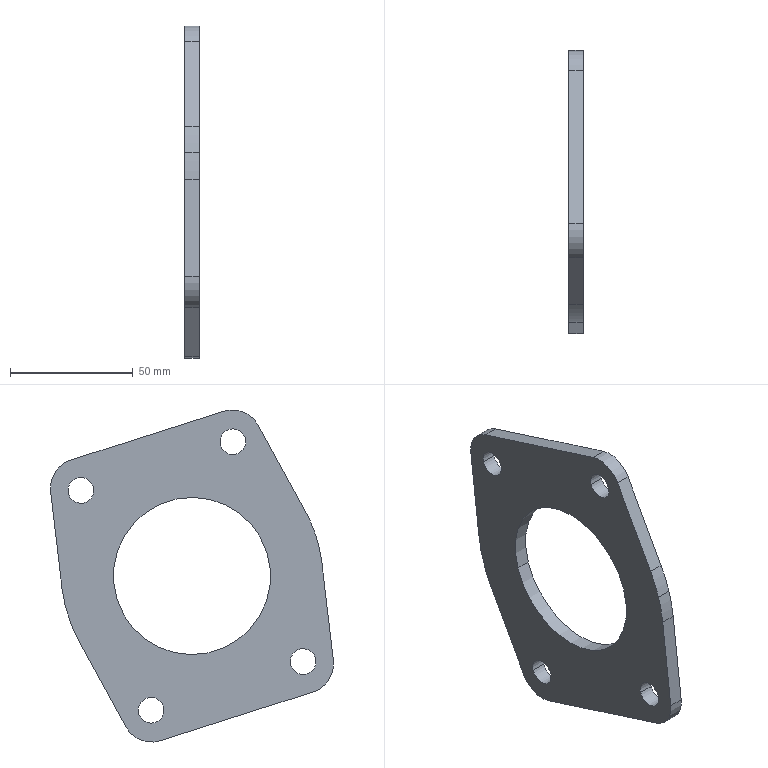Part | NX | features BREP 1 | 1 solid | 25 faces | box 6 x 115.344 x 135.296 mm | volume 47647 mm3 | cylinder 17 | plane 8 | commonest cylinder face diameters 10.5 x8 24 x4 120 x3 64 x2
STEP:
#1=CARTESIAN_POINT('',(-624.265,-30.481,9.741));
#2=VERTEX_POINT('',#1);
#3=CARTESIAN_POINT('',(-624.265,30.481,-9.741));
#4=VERTEX_POINT('',#3);
#5=CARTESIAN_POINT('',(-624.265,0.,0.));
#6=DIRECTION('',(1.,0.,0.));
#7=DIRECTION('',(0.,-0.9525,0.3044));
#8=AXIS2_PLACEMENT_3D('',#5,#6,#7);
#9=CIRCLE('',#8,32.);
#10=EDGE_CURVE('',#2,#4,#9,.T.);
#11=ORIENTED_EDGE('',*,*,#10,.T.);
#12=CARTESIAN_POINT('',(-630.265,30.481,-9.741));
#13=VERTEX_POINT('',#12);
#14=CARTESIAN_POINT('',(-624.265,30.481,-9.741));
#15=DIRECTION('',(-1.,0.,0.));
#16=VECTOR('',#15,1000.);
#17=LINE('',#14,#16);
#18=EDGE_CURVE('',#13,#4,#17,.F.);
#19=ORIENTED_EDGE('',*,*,#18,.F.);
#20=CARTESIAN_POINT('',(-630.265,-30.481,9.741));
#21=VERTEX_POINT('',#20);
#22=CARTESIAN_POINT('',(-630.265,0.,0.));
#23=DIRECTION('',(1.,0.,0.));
#24=DIRECTION('',(0.,-0.9525,0.3044));
#25=AXIS2_PLACEMENT_3D('',#22,#23,#24);
#26=CIRCLE('',#25,32.);
#27=EDGE_CURVE('',#21,#13,#26,.T.);
#28=ORIENTED_EDGE('',*,*,#27,.F.);
#29=CARTESIAN_POINT('',(-624.265,-30.481,9.741));
#30=DIRECTION('',(-1.,0.,0.));
#31=VECTOR('',#30,1000.);
#32=LINE('',#29,#31);
#33=EDGE_CURVE('',#21,#2,#32,.F.);
#34=ORIENTED_EDGE('',*,*,#33,.T.);
#35=EDGE_LOOP('',(#11,#19,#28,#34));
#36=FACE_BOUND('',#35,.T.);
#37=CARTESIAN_POINT('',(-624.265,0.,0.));
#38=DIRECTION('',(-1.,0.,0.));
#39=DIRECTION('',(0.,0.9525,-0.3044));
#40=AXIS2_PLACEMENT_3D('',#37,#38,#39);
#41=CYLINDRICAL_SURFACE('',#40,32.);
#42=ADVANCED_FACE('',(#36),#41,.F.);
#43=CARTESIAN_POINT('',(-624.265,40.264,36.474));
#44=VERTEX_POINT('',#43);
#45=CARTESIAN_POINT('',(-624.265,50.266,33.278));
#46=VERTEX_POINT('',#45);
#47=CARTESIAN_POINT('',(-624.265,45.265,34.876));
#48=DIRECTION('',(1.,0.,0.));
#49=DIRECTION('',(0.,-0.9525,0.3044));
#50=AXIS2_PLACEMENT_3D('',#47,#48,#49);
#51=CIRCLE('',#50,5.25);
#52=EDGE_CURVE('',#44,#46,#51,.T.);
#53=ORIENTED_EDGE('',*,*,#52,.T.);
#54=CARTESIAN_POINT('',(-630.265,50.266,33.278));
#55=VERTEX_POINT('',#54);
#56=CARTESIAN_POINT('',(-624.265,50.266,33.278));
#57=DIRECTION('',(-1.,0.,0.));
#58=VECTOR('',#57,1000.);
#59=LINE('',#56,#58);
#60=EDGE_CURVE('',#55,#46,#59,.F.);
#61=ORIENTED_EDGE('',*,*,#60,.F.);
#62=CARTESIAN_POINT('',(-630.265,40.264,36.474));
#63=VERTEX_POINT('',#62);
#64=CARTESIAN_POINT('',(-630.265,45.265,34.876));
#65=DIRECTION('',(1.,0.,0.));
#66=DIRECTION('',(0.,-0.9525,0.3044));
#67=AXIS2_PLACEMENT_3D('',#64,#65,#66);
#68=CIRCLE('',#67,5.25);
#69=EDGE_CURVE('',#63,#55,#68,.T.);
#70=ORIENTED_EDGE('',*,*,#69,.F.);
#71=CARTESIAN_POINT('',(-624.265,40.264,36.474));
#72=DIRECTION('',(-1.,0.,0.));
#73=VECTOR('',#72,1000.);
#74=LINE('',#71,#73);
#75=EDGE_CURVE('',#63,#44,#74,.F.);
#76=ORIENTED_EDGE('',*,*,#75,.T.);
#77=EDGE_LOOP('',(#53,#61,#70,#76));
#78=FACE_BOUND('',#77,.T.);
#79=CARTESIAN_POINT('',(-624.265,45.265,34.876));
#80=DIRECTION('',(-1.,0.,0.));
#81=DIRECTION('',(0.,0.9525,-0.3044));
#82=AXIS2_PLACEMENT_3D('',#79,#80,#81);
#83=CYLINDRICAL_SURFACE('',#82,5.25);
#84=ADVANCED_FACE('',(#78),#83,.F.);
#85=CARTESIAN_POINT('',(-624.265,-21.651,56.261));
#86=VERTEX_POINT('',#85);
#87=CARTESIAN_POINT('',(-624.265,-11.65,53.065));
#88=VERTEX_POINT('',#87);
#89=CARTESIAN_POINT('',(-624.265,-16.65,54.663));
#90=DIRECTION('',(1.,0.,0.));
#91=DIRECTION('',(0.,-0.9525,0.3044));
#92=AXIS2_PLACEMENT_3D('',#89,#90,#91);
#93=CIRCLE('',#92,5.25);
#94=EDGE_CURVE('',#86,#88,#93,.T.);
#95=ORIENTED_EDGE('',*,*,#94,.T.);
#96=CARTESIAN_POINT('',(-630.265,-11.65,53.065));
#97=VERTEX_POINT('',#96);
#98=CARTESIAN_POINT('',(-624.265,-11.65,53.065));
#99=DIRECTION('',(-1.,0.,0.));
#100=VECTOR('',#99,1000.);
#101=LINE('',#98,#100);
#102=EDGE_CURVE('',#97,#88,#101,.F.);
#103=ORIENTED_EDGE('',*,*,#102,.F.);
#104=CARTESIAN_POINT('',(-630.265,-21.651,56.261));
#105=VERTEX_POINT('',#104);
#106=CARTESIAN_POINT('',(-630.265,-16.65,54.663));
#107=DIRECTION('',(1.,0.,0.));
#108=DIRECTION('',(0.,-0.9525,0.3044));
#109=AXIS2_PLACEMENT_3D('',#106,#107,#108);
#110=CIRCLE('',#109,5.25);
#111=EDGE_CURVE('',#105,#97,#110,.T.);
#112=ORIENTED_EDGE('',*,*,#111,.F.);
#113=CARTESIAN_POINT('',(-624.265,-21.651,56.261));
#114=DIRECTION('',(-1.,0.,0.));
#115=VECTOR('',#114,1000.);
#116=LINE('',#113,#115);
#117=EDGE_CURVE('',#105,#86,#116,.F.);
#118=ORIENTED_EDGE('',*,*,#117,.T.);
#119=EDGE_LOOP('',(#95,#103,#112,#118));
#120=FACE_BOUND('',#119,.T.);
#121=CARTESIAN_POINT('',(-624.265,-16.65,54.663));
#122=DIRECTION('',(-1.,0.,0.));
#123=DIRECTION('',(0.,0.9525,-0.3044));
#124=AXIS2_PLACEMENT_3D('',#121,#122,#123);
#125=CYLINDRICAL_SURFACE('',#124,5.25);
#126=ADVANCED_FACE('',(#120),#125,.F.);
#127=CARTESIAN_POINT('',(-624.265,-50.266,-33.278));
#128=VERTEX_POINT('',#127);
#129=CARTESIAN_POINT('',(-624.265,-40.264,-36.474));
#130=VERTEX_POINT('',#129);
#131=CARTESIAN_POINT('',(-624.265,-45.265,-34.876));
#132=DIRECTION('',(1.,0.,0.));
#133=DIRECTION('',(0.,-0.9525,0.3044));
#134=AXIS2_PLACEMENT_3D('',#131,#132,#133);
#135=CIRCLE('',#134,5.25);
#136=EDGE_CURVE('',#128,#130,#135,.T.);
#137=ORIENTED_EDGE('',*,*,#136,.T.);
#138=CARTESIAN_POINT('',(-630.265,-40.264,-36.474));
#139=VERTEX_POINT('',#138);
#140=CARTESIAN_POINT('',(-624.265,-40.264,-36.474));
#141=DIRECTION('',(-1.,0.,0.));
#142=VECTOR('',#141,1000.);
#143=LINE('',#140,#142);
#144=EDGE_CURVE('',#139,#130,#143,.F.);
#145=ORIENTED_EDGE('',*,*,#144,.F.);
#146=CARTESIAN_POINT('',(-630.265,-50.266,-33.278));
#147=VERTEX_POINT('',#146);
#148=CARTESIAN_POINT('',(-630.265,-45.265,-34.876));
#149=DIRECTION('',(1.,0.,0.));
#150=DIRECTION('',(0.,-0.9525,0.3044));
#151=AXIS2_PLACEMENT_3D('',#148,#149,#150);
#152=CIRCLE('',#151,5.25);
#153=EDGE_CURVE('',#147,#139,#152,.T.);
#154=ORIENTED_EDGE('',*,*,#153,.F.);
#155=CARTESIAN_POINT('',(-624.265,-50.266,-33.278));
#156=DIRECTION('',(-1.,0.,0.));
#157=VECTOR('',#156,1000.);
#158=LINE('',#155,#157);
#159=EDGE_CURVE('',#147,#128,#158,.F.);
#160=ORIENTED_EDGE('',*,*,#159,.T.);
#161=EDGE_LOOP('',(#137,#145,#154,#160));
#162=FACE_BOUND('',#161,.T.);
#163=CARTESIAN_POINT('',(-624.265,-45.265,-34.876));
#164=DIRECTION('',(-1.,0.,0.));
#165=DIRECTION('',(0.,0.9525,-0.3044));
#166=AXIS2_PLACEMENT_3D('',#163,#164,#165);
#167=CYLINDRICAL_SURFACE('',#166,5.25);
#168=ADVANCED_FACE('',(#162),#167,.F.);
#169=CARTESIAN_POINT('',(-624.265,11.65,-53.065));
#170=VERTEX_POINT('',#169);
#171=CARTESIAN_POINT('',(-624.265,21.651,-56.261));
#172=VERTEX_POINT('',#171);
#173=CARTESIAN_POINT('',(-624.265,16.65,-54.663));
#174=DIRECTION('',(1.,0.,0.));
#175=DIRECTION('',(0.,-0.9525,0.3044));
#176=AXIS2_PLACEMENT_3D('',#173,#174,#175);
#177=CIRCLE('',#176,5.25);
#178=EDGE_CURVE('',#170,#172,#177,.T.);
#179=ORIENTED_EDGE('',*,*,#178,.T.);
#180=CARTESIAN_POINT('',(-630.265,21.651,-56.261));
#181=VERTEX_POINT('',#180);
#182=CARTESIAN_POINT('',(-624.265,21.651,-56.261));
#183=DIRECTION('',(-1.,0.,0.));
#184=VECTOR('',#183,1000.);
#185=LINE('',#182,#184);
#186=EDGE_CURVE('',#181,#172,#185,.F.);
#187=ORIENTED_EDGE('',*,*,#186,.F.);
#188=CARTESIAN_POINT('',(-630.265,11.65,-53.065));
#189=VERTEX_POINT('',#188);
#190=CARTESIAN_POINT('',(-630.265,16.65,-54.663));
#191=DIRECTION('',(1.,0.,0.));
#192=DIRECTION('',(0.,-0.9525,0.3044));
#193=AXIS2_PLACEMENT_3D('',#190,#191,#192);
#194=CIRCLE('',#193,5.25);
#195=EDGE_CURVE('',#189,#181,#194,.T.);
#196=ORIENTED_EDGE('',*,*,#195,.F.);
#197=CARTESIAN_POINT('',(-624.265,11.65,-53.065));
#198=DIRECTION('',(-1.,0.,0.));
#199=VECTOR('',#198,1000.);
#200=LINE('',#197,#199);
#201=EDGE_CURVE('',#189,#170,#200,.F.);
#202=ORIENTED_EDGE('',*,*,#201,.T.);
#203=EDGE_LOOP('',(#179,#187,#196,#202));
#204=FACE_BOUND('',#203,.T.);
#205=CARTESIAN_POINT('',(-624.265,16.65,-54.663));
#206=DIRECTION('',(-1.,0.,0.));
#207=DIRECTION('',(0.,0.9525,-0.3044));
#208=AXIS2_PLACEMENT_3D('',#205,#206,#207);
#209=CYLINDRICAL_SURFACE('',#208,5.25);
#210=ADVANCED_FACE('',(#204),#209,.F.);
#211=CARTESIAN_POINT('',(-624.265,-50.523,16.146));
#212=VERTEX_POINT('',#211);
#213=CARTESIAN_POINT('',(-624.265,-52.958,4.905));
#214=VERTEX_POINT('',#213);
#215=CARTESIAN_POINT('',(-624.265,6.63,-2.119));
#216=DIRECTION('',(1.,0.,0.));
#217=DIRECTION('',(0.,0.9525,-0.3044));
#218=AXIS2_PLACEMENT_3D('',#215,#216,#217);
#219=CIRCLE('',#218,60.);
#220=EDGE_CURVE('',#212,#214,#219,.T.);
#221=ORIENTED_EDGE('',*,*,#220,.F.);
#222=CARTESIAN_POINT('',(-630.265,-50.523,16.146));
#223=VERTEX_POINT('',#222);
#224=CARTESIAN_POINT('',(-624.265,-50.523,16.146));
#225=DIRECTION('',(-1.,0.,0.));
#226=VECTOR('',#225,1000.);
#227=LINE('',#224,#226);
#228=EDGE_CURVE('',#212,#223,#227,.T.);
#229=ORIENTED_EDGE('',*,*,#228,.T.);
#230=CARTESIAN_POINT('',(-630.265,-52.958,4.905));
#231=VERTEX_POINT('',#230);
#232=CARTESIAN_POINT('',(-630.265,6.63,-2.119));
#233=DIRECTION('',(1.,0.,0.));
#234=DIRECTION('',(0.,0.9525,-0.3044));
#235=AXIS2_PLACEMENT_3D('',#232,#233,#234);
#236=CIRCLE('',#235,60.);
#237=EDGE_CURVE('',#223,#231,#236,.T.);
#238=ORIENTED_EDGE('',*,*,#237,.T.);
#239=CARTESIAN_POINT('',(-624.265,-52.958,4.905));
#240=DIRECTION('',(-1.,0.,0.));
#241=VECTOR('',#240,1000.);
#242=LINE('',#239,#241);
#243=EDGE_CURVE('',#214,#231,#242,.T.);
#244=ORIENTED_EDGE('',*,*,#243,.F.);
#245=EDGE_LOOP('',(#221,#229,#238,#244));
#246=FACE_BOUND('',#245,.T.);
#247=CARTESIAN_POINT('',(-624.265,6.63,-2.119));
#248=DIRECTION('',(-1.,0.,0.));
#249=DIRECTION('',(0.,0.9525,-0.3044));
#250=AXIS2_PLACEMENT_3D('',#247,#248,#249);
#251=CYLINDRICAL_SURFACE('',#250,60.);
#252=ADVANCED_FACE('',(#246),#251,.T.);
#253=ORIENTED_EDGE('',*,*,#52,.F.);
#254=CARTESIAN_POINT('',(-624.265,45.265,34.876));
#255=DIRECTION('',(1.,0.,0.));
#256=DIRECTION('',(0.,-0.9525,0.3044));
#257=AXIS2_PLACEMENT_3D('',#254,#255,#256);
#258=CIRCLE('',#257,5.25);
#259=EDGE_CURVE('',#46,#44,#258,.T.);
#260=ORIENTED_EDGE('',*,*,#259,.F.);
#261=EDGE_LOOP('',(#253,#260));
#262=FACE_BOUND('',#261,.T.);
#263=ORIENTED_EDGE('',*,*,#136,.F.);
#264=CARTESIAN_POINT('',(-624.265,-45.265,-34.876));
#265=DIRECTION('',(1.,0.,0.));
#266=DIRECTION('',(0.,-0.9525,0.3044));
#267=AXIS2_PLACEMENT_3D('',#264,#265,#266);
#268=CIRCLE('',#267,5.25);
#269=EDGE_CURVE('',#130,#128,#268,.T.);
#270=ORIENTED_EDGE('',*,*,#269,.F.);
#271=EDGE_LOOP('',(#263,#270));
#272=FACE_BOUND('',#271,.T.);
#273=CARTESIAN_POINT('',(-624.265,-57.59,-34.391));
#274=VERTEX_POINT('',#273);
#275=CARTESIAN_POINT('',(-624.265,-49.325,-47.226));
#276=VERTEX_POINT('',#275);
#277=CARTESIAN_POINT('',(-624.265,-45.672,-35.796));
#278=DIRECTION('',(1.,0.,0.));
#279=DIRECTION('',(0.,0.9525,-0.3044));
#280=AXIS2_PLACEMENT_3D('',#277,#278,#279);
#281=CIRCLE('',#280,12.);
#282=EDGE_CURVE('',#274,#276,#281,.T.);
#283=ORIENTED_EDGE('',*,*,#282,.T.);
#284=CARTESIAN_POINT('',(-624.265,12.796,-67.079));
#285=VERTEX_POINT('',#284);
#286=CARTESIAN_POINT('',(-624.265,-49.325,-47.226));
#287=DIRECTION('',(0.,0.9525,-0.3044));
#288=VECTOR('',#287,1000.);
#289=LINE('',#286,#288);
#290=EDGE_CURVE('',#276,#285,#289,.T.);
#291=ORIENTED_EDGE('',*,*,#290,.T.);
#292=CARTESIAN_POINT('',(-624.265,26.972,-61.415));
#293=VERTEX_POINT('',#292);
#294=CARTESIAN_POINT('',(-624.265,16.449,-55.648));
#295=DIRECTION('',(1.,0.,0.));
#296=DIRECTION('',(0.,0.9525,-0.3044));
#297=AXIS2_PLACEMENT_3D('',#294,#295,#296);
#298=CIRCLE('',#297,12.);
#299=EDGE_CURVE('',#285,#293,#298,.T.);
#300=ORIENTED_EDGE('',*,*,#299,.T.);
#301=CARTESIAN_POINT('',(-624.265,45.988,-26.715));
#302=VERTEX_POINT('',#301);
#303=CARTESIAN_POINT('',(-624.265,26.972,-61.415));
#304=DIRECTION('',(0.,0.4806,0.877));
#305=VECTOR('',#304,1000.);
#306=LINE('',#303,#305);
#307=EDGE_CURVE('',#293,#302,#306,.T.);
#308=ORIENTED_EDGE('',*,*,#307,.T.);
#309=CARTESIAN_POINT('',(-624.265,52.958,-4.905));
#310=VERTEX_POINT('',#309);
#311=CARTESIAN_POINT('',(-624.265,-6.63,2.119));
#312=DIRECTION('',(1.,0.,0.));
#313=DIRECTION('',(0.,0.9525,-0.3044));
#314=AXIS2_PLACEMENT_3D('',#311,#312,#313);
#315=CIRCLE('',#314,60.);
#316=EDGE_CURVE('',#302,#310,#315,.T.);
#317=ORIENTED_EDGE('',*,*,#316,.T.);
#318=CARTESIAN_POINT('',(-624.265,57.59,34.391));
#319=VERTEX_POINT('',#318);
#320=CARTESIAN_POINT('',(-624.265,52.958,-4.905));
#321=DIRECTION('',(0.,0.1171,0.9931));
#322=VECTOR('',#321,1000.);
#323=LINE('',#320,#322);
#324=EDGE_CURVE('',#310,#319,#323,.T.);
#325=ORIENTED_EDGE('',*,*,#324,.T.);
#326=CARTESIAN_POINT('',(-624.265,49.325,47.226));
#327=VERTEX_POINT('',#326);
#328=CARTESIAN_POINT('',(-624.265,45.672,35.796));
#329=DIRECTION('',(1.,0.,0.));
#330=DIRECTION('',(0.,0.9525,-0.3044));
#331=AXIS2_PLACEMENT_3D('',#328,#329,#330);
#332=CIRCLE('',#331,12.);
#333=EDGE_CURVE('',#319,#327,#332,.T.);
#334=ORIENTED_EDGE('',*,*,#333,.T.);
#335=CARTESIAN_POINT('',(-624.265,-12.796,67.079));
#336=VERTEX_POINT('',#335);
#337=CARTESIAN_POINT('',(-624.265,49.325,47.226));
#338=DIRECTION('',(0.,-0.9525,0.3044));
#339=VECTOR('',#338,1000.);
#340=LINE('',#337,#339);
#341=EDGE_CURVE('',#327,#336,#340,.T.);
#342=ORIENTED_EDGE('',*,*,#341,.T.);
#343=CARTESIAN_POINT('',(-624.265,-26.972,61.415));
#344=VERTEX_POINT('',#343);
#345=CARTESIAN_POINT('',(-624.265,-16.449,55.648));
#346=DIRECTION('',(1.,0.,0.));
#347=DIRECTION('',(0.,0.9525,-0.3044));
#348=AXIS2_PLACEMENT_3D('',#345,#346,#347);
#349=CIRCLE('',#348,12.);
#350=EDGE_CURVE('',#336,#344,#349,.T.);
#351=ORIENTED_EDGE('',*,*,#350,.T.);
#352=CARTESIAN_POINT('',(-624.265,-45.988,26.715));
#353=VERTEX_POINT('',#352);
#354=CARTESIAN_POINT('',(-624.265,-26.972,61.415));
#355=DIRECTION('',(0.,-0.4806,-0.877));
#356=VECTOR('',#355,1000.);
#357=LINE('',#354,#356);
#358=EDGE_CURVE('',#344,#353,#357,.T.);
#359=ORIENTED_EDGE('',*,*,#358,.T.);
#360=CARTESIAN_POINT('',(-624.265,6.63,-2.119));
#361=DIRECTION('',(1.,0.,0.));
#362=DIRECTION('',(0.,0.9525,-0.3044));
#363=AXIS2_PLACEMENT_3D('',#360,#361,#362);
#364=CIRCLE('',#363,60.);
#365=EDGE_CURVE('',#353,#212,#364,.T.);
#366=ORIENTED_EDGE('',*,*,#365,.T.);
#367=ORIENTED_EDGE('',*,*,#220,.T.);
#368=CARTESIAN_POINT('',(-624.265,-52.958,4.905));
#369=DIRECTION('',(0.,-0.1171,-0.9931));
#370=VECTOR('',#369,1000.);
#371=LINE('',#368,#370);
#372=EDGE_CURVE('',#214,#274,#371,.T.);
#373=ORIENTED_EDGE('',*,*,#372,.T.);
#374=EDGE_LOOP('',(#283,#291,#300,#308,#317,#325,#334,#342,#351,#359,#366,#367,#373));
#375=FACE_BOUND('',#374,.T.);
#376=ORIENTED_EDGE('',*,*,#178,.F.);
#377=CARTESIAN_POINT('',(-624.265,16.65,-54.663));
#378=DIRECTION('',(1.,0.,0.));
#379=DIRECTION('',(0.,-0.9525,0.3044));
#380=AXIS2_PLACEMENT_3D('',#377,#378,#379);
#381=CIRCLE('',#380,5.25);
#382=EDGE_CURVE('',#172,#170,#381,.T.);
#383=ORIENTED_EDGE('',*,*,#382,.F.);
#384=EDGE_LOOP('',(#376,#383));
#385=FACE_BOUND('',#384,.T.);
#386=ORIENTED_EDGE('',*,*,#94,.F.);
#387=CARTESIAN_POINT('',(-624.265,-16.65,54.663));
#388=DIRECTION('',(1.,0.,0.));
#389=DIRECTION('',(0.,-0.9525,0.3044));
#390=AXIS2_PLACEMENT_3D('',#387,#388,#389);
#391=CIRCLE('',#390,5.25);
#392=EDGE_CURVE('',#88,#86,#391,.T.);
#393=ORIENTED_EDGE('',*,*,#392,.F.);
#394=EDGE_LOOP('',(#386,#393));
#395=FACE_BOUND('',#394,.T.);
#396=ORIENTED_EDGE('',*,*,#10,.F.);
#397=CARTESIAN_POINT('',(-624.265,0.,0.));
#398=DIRECTION('',(1.,0.,0.));
#399=DIRECTION('',(0.,-0.9525,0.3044));
#400=AXIS2_PLACEMENT_3D('',#397,#398,#399);
#401=CIRCLE('',#400,32.);
#402=EDGE_CURVE('',#4,#2,#401,.T.);
#403=ORIENTED_EDGE('',*,*,#402,.F.);
#404=EDGE_LOOP('',(#396,#403));
#405=FACE_BOUND('',#404,.T.);
#406=CARTESIAN_POINT('',(-624.265,-45.672,-35.796));
#407=DIRECTION('',(1.,0.,0.));
#408=DIRECTION('',(0.,-0.9525,0.3044));
#409=AXIS2_PLACEMENT_3D('',#406,#407,#408);
#410=PLANE('',#409);
#411=ADVANCED_FACE('',(#262,#272,#375,#385,#395,#405),#410,.T.);
#412=CARTESIAN_POINT('',(-630.265,-57.59,-34.391));
#413=VERTEX_POINT('',#412);
#414=CARTESIAN_POINT('',(-630.265,-49.325,-47.226));
#415=VERTEX_POINT('',#414);
#416=CARTESIAN_POINT('',(-630.265,-45.672,-35.796));
#417=DIRECTION('',(1.,0.,0.));
#418=DIRECTION('',(0.,0.9525,-0.3044));
#419=AXIS2_PLACEMENT_3D('',#416,#417,#418);
#420=CIRCLE('',#419,12.);
#421=EDGE_CURVE('',#413,#415,#420,.T.);
#422=ORIENTED_EDGE('',*,*,#421,.F.);
#423=CARTESIAN_POINT('',(-630.265,-52.958,4.905));
#424=DIRECTION('',(0.,-0.1171,-0.9931));
#425=VECTOR('',#424,1000.);
#426=LINE('',#423,#425);
#427=EDGE_CURVE('',#231,#413,#426,.T.);
#428=ORIENTED_EDGE('',*,*,#427,.F.);
#429=ORIENTED_EDGE('',*,*,#237,.F.);
#430=CARTESIAN_POINT('',(-630.265,-45.988,26.715));
#431=VERTEX_POINT('',#430);
#432=CARTESIAN_POINT('',(-630.265,6.63,-2.119));
#433=DIRECTION('',(1.,0.,0.));
#434=DIRECTION('',(0.,0.9525,-0.3044));
#435=AXIS2_PLACEMENT_3D('',#432,#433,#434);
#436=CIRCLE('',#435,60.);
#437=EDGE_CURVE('',#431,#223,#436,.T.);
#438=ORIENTED_EDGE('',*,*,#437,.F.);
#439=CARTESIAN_POINT('',(-630.265,-26.972,61.415));
#440=VERTEX_POINT('',#439);
#441=CARTESIAN_POINT('',(-630.265,-26.972,61.415));
#442=DIRECTION('',(0.,-0.4806,-0.877));
#443=VECTOR('',#442,1000.);
#444=LINE('',#441,#443);
#445=EDGE_CURVE('',#440,#431,#444,.T.);
#446=ORIENTED_EDGE('',*,*,#445,.F.);
#447=CARTESIAN_POINT('',(-630.265,-12.796,67.079));
#448=VERTEX_POINT('',#447);
#449=CARTESIAN_POINT('',(-630.265,-16.449,55.648));
#450=DIRECTION('',(1.,0.,0.));
#451=DIRECTION('',(0.,0.9525,-0.3044));
#452=AXIS2_PLACEMENT_3D('',#449,#450,#451);
#453=CIRCLE('',#452,12.);
#454=EDGE_CURVE('',#448,#440,#453,.T.);
#455=ORIENTED_EDGE('',*,*,#454,.F.);
#456=CARTESIAN_POINT('',(-630.265,49.325,47.226));
#457=VERTEX_POINT('',#456);
#458=CARTESIAN_POINT('',(-630.265,49.325,47.226));
#459=DIRECTION('',(0.,-0.9525,0.3044));
#460=VECTOR('',#459,1000.);
#461=LINE('',#458,#460);
#462=EDGE_CURVE('',#457,#448,#461,.T.);
#463=ORIENTED_EDGE('',*,*,#462,.F.);
#464=CARTESIAN_POINT('',(-630.265,57.59,34.391));
#465=VERTEX_POINT('',#464);
#466=CARTESIAN_POINT('',(-630.265,45.672,35.796));
#467=DIRECTION('',(1.,0.,0.));
#468=DIRECTION('',(0.,0.9525,-0.3044));
#469=AXIS2_PLACEMENT_3D('',#466,#467,#468);
#470=CIRCLE('',#469,12.);
#471=EDGE_CURVE('',#465,#457,#470,.T.);
#472=ORIENTED_EDGE('',*,*,#471,.F.);
#473=CARTESIAN_POINT('',(-630.265,52.958,-4.905));
#474=VERTEX_POINT('',#473);
#475=CARTESIAN_POINT('',(-630.265,52.958,-4.905));
#476=DIRECTION('',(0.,0.1171,0.9931));
#477=VECTOR('',#476,1000.);
#478=LINE('',#475,#477);
#479=EDGE_CURVE('',#474,#465,#478,.T.);
#480=ORIENTED_EDGE('',*,*,#479,.F.);
#481=CARTESIAN_POINT('',(-630.265,45.988,-26.715));
#482=VERTEX_POINT('',#481);
#483=CARTESIAN_POINT('',(-630.265,-6.63,2.119));
#484=DIRECTION('',(1.,0.,0.));
#485=DIRECTION('',(0.,0.9525,-0.3044));
#486=AXIS2_PLACEMENT_3D('',#483,#484,#485);
#487=CIRCLE('',#486,60.);
#488=EDGE_CURVE('',#482,#474,#487,.T.);
#489=ORIENTED_EDGE('',*,*,#488,.F.);
#490=CARTESIAN_POINT('',(-630.265,26.972,-61.415));
#491=VERTEX_POINT('',#490);
#492=CARTESIAN_POINT('',(-630.265,26.972,-61.415));
#493=DIRECTION('',(0.,0.4806,0.877));
#494=VECTOR('',#493,1000.);
#495=LINE('',#492,#494);
#496=EDGE_CURVE('',#491,#482,#495,.T.);
#497=ORIENTED_EDGE('',*,*,#496,.F.);
#498=CARTESIAN_POINT('',(-630.265,12.796,-67.079));
#499=VERTEX_POINT('',#498);
#500=CARTESIAN_POINT('',(-630.265,16.449,-55.648));
#501=DIRECTION('',(1.,0.,0.));
#502=DIRECTION('',(0.,0.9525,-0.3044));
#503=AXIS2_PLACEMENT_3D('',#500,#501,#502);
#504=CIRCLE('',#503,12.);
#505=EDGE_CURVE('',#499,#491,#504,.T.);
#506=ORIENTED_EDGE('',*,*,#505,.F.);
#507=CARTESIAN_POINT('',(-630.265,-49.325,-47.226));
#508=DIRECTION('',(0.,0.9525,-0.3044));
#509=VECTOR('',#508,1000.);
#510=LINE('',#507,#509);
#511=EDGE_CURVE('',#415,#499,#510,.T.);
#512=ORIENTED_EDGE('',*,*,#511,.F.);
#513=EDGE_LOOP('',(#422,#428,#429,#438,#446,#455,#463,#472,#480,#489,#497,#506,#512));
#514=FACE_BOUND('',#513,.T.);
#515=ORIENTED_EDGE('',*,*,#195,.T.);
#516=CARTESIAN_POINT('',(-630.265,16.65,-54.663));
#517=DIRECTION('',(1.,0.,0.));
#518=DIRECTION('',(0.,-0.9525,0.3044));
#519=AXIS2_PLACEMENT_3D('',#516,#517,#518);
#520=CIRCLE('',#519,5.25);
#521=EDGE_CURVE('',#181,#189,#520,.T.);
#522=ORIENTED_EDGE('',*,*,#521,.T.);
#523=EDGE_LOOP('',(#515,#522));
#524=FACE_BOUND('',#523,.T.);
#525=ORIENTED_EDGE('',*,*,#153,.T.);
#526=CARTESIAN_POINT('',(-630.265,-45.265,-34.876));
#527=DIRECTION('',(1.,0.,0.));
#528=DIRECTION('',(0.,-0.9525,0.3044));
#529=AXIS2_PLACEMENT_3D('',#526,#527,#528);
#530=CIRCLE('',#529,5.25);
#531=EDGE_CURVE('',#139,#147,#530,.T.);
#532=ORIENTED_EDGE('',*,*,#531,.T.);
#533=EDGE_LOOP('',(#525,#532));
#534=FACE_BOUND('',#533,.T.);
#535=ORIENTED_EDGE('',*,*,#111,.T.);
#536=CARTESIAN_POINT('',(-630.265,-16.65,54.663));
#537=DIRECTION('',(1.,0.,0.));
#538=DIRECTION('',(0.,-0.9525,0.3044));
#539=AXIS2_PLACEMENT_3D('',#536,#537,#538);
#540=CIRCLE('',#539,5.25);
#541=EDGE_CURVE('',#97,#105,#540,.T.);
#542=ORIENTED_EDGE('',*,*,#541,.T.);
#543=EDGE_LOOP('',(#535,#542));
#544=FACE_BOUND('',#543,.T.);
#545=ORIENTED_EDGE('',*,*,#69,.T.);
#546=CARTESIAN_POINT('',(-630.265,45.265,34.876));
#547=DIRECTION('',(1.,0.,0.));
#548=DIRECTION('',(0.,-0.9525,0.3044));
#549=AXIS2_PLACEMENT_3D('',#546,#547,#548);
#550=CIRCLE('',#549,5.25);
#551=EDGE_CURVE('',#55,#63,#550,.T.);
#552=ORIENTED_EDGE('',*,*,#551,.T.);
#553=EDGE_LOOP('',(#545,#552));
#554=FACE_BOUND('',#553,.T.);
#555=ORIENTED_EDGE('',*,*,#27,.T.);
#556=CARTESIAN_POINT('',(-630.265,0.,0.));
#557=DIRECTION('',(1.,0.,0.));
#558=DIRECTION('',(0.,-0.9525,0.3044));
#559=AXIS2_PLACEMENT_3D('',#556,#557,#558);
#560=CIRCLE('',#559,32.);
#561=EDGE_CURVE('',#13,#21,#560,.T.);
#562=ORIENTED_EDGE('',*,*,#561,.T.);
#563=EDGE_LOOP('',(#555,#562));
#564=FACE_BOUND('',#563,.T.);
#565=CARTESIAN_POINT('',(-630.265,-45.672,-35.796));
#566=DIRECTION('',(1.,0.,0.));
#567=DIRECTION('',(0.,-0.9525,0.3044));
#568=AXIS2_PLACEMENT_3D('',#565,#566,#567);
#569=PLANE('',#568);
#570=ADVANCED_FACE('',(#514,#524,#534,#544,#554,#564),#569,.F.);
#571=ORIENTED_EDGE('',*,*,#421,.T.);
#572=CARTESIAN_POINT('',(-624.265,-49.325,-47.226));
#573=DIRECTION('',(-1.,0.,0.));
#574=VECTOR('',#573,1000.);
#575=LINE('',#572,#574);
#576=EDGE_CURVE('',#276,#415,#575,.T.);
#577=ORIENTED_EDGE('',*,*,#576,.F.);
#578=ORIENTED_EDGE('',*,*,#282,.F.);
#579=CARTESIAN_POINT('',(-624.265,-57.59,-34.391));
#580=DIRECTION('',(-1.,0.,0.));
#581=VECTOR('',#580,1000.);
#582=LINE('',#579,#581);
#583=EDGE_CURVE('',#274,#413,#582,.T.);
#584=ORIENTED_EDGE('',*,*,#583,.T.);
#585=EDGE_LOOP('',(#571,#577,#578,#584));
#586=FACE_BOUND('',#585,.T.);
#587=CARTESIAN_POINT('',(-624.265,-45.672,-35.796));
#588=DIRECTION('',(-1.,0.,0.));
#589=DIRECTION('',(0.,0.9525,-0.3044));
#590=AXIS2_PLACEMENT_3D('',#587,#588,#589);
#591=CYLINDRICAL_SURFACE('',#590,12.);
#592=ADVANCED_FACE('',(#586),#591,.T.);
#593=ORIENTED_EDGE('',*,*,#511,.T.);
#594=CARTESIAN_POINT('',(-624.265,12.796,-67.079));
#595=DIRECTION('',(-1.,0.,0.));
#596=VECTOR('',#595,1000.);
#597=LINE('',#594,#596);
#598=EDGE_CURVE('',#285,#499,#597,.T.);
#599=ORIENTED_EDGE('',*,*,#598,.F.);
#600=ORIENTED_EDGE('',*,*,#290,.F.);
#601=ORIENTED_EDGE('',*,*,#576,.T.);
#602=EDGE_LOOP('',(#593,#599,#600,#601));
#603=FACE_BOUND('',#602,.T.);
#604=CARTESIAN_POINT('',(-624.265,-49.325,-47.226));
#605=DIRECTION('',(0.,0.3044,0.9525));
#606=DIRECTION('',(0.,0.9525,-0.3044));
#607=AXIS2_PLACEMENT_3D('',#604,#605,#606);
#608=PLANE('',#607);
#609=ADVANCED_FACE('',(#603),#608,.F.);
#610=ORIENTED_EDGE('',*,*,#505,.T.);
#611=CARTESIAN_POINT('',(-624.265,26.972,-61.415));
#612=DIRECTION('',(-1.,0.,0.));
#613=VECTOR('',#612,1000.);
#614=LINE('',#611,#613);
#615=EDGE_CURVE('',#293,#491,#614,.T.);
#616=ORIENTED_EDGE('',*,*,#615,.F.);
#617=ORIENTED_EDGE('',*,*,#299,.F.);
#618=ORIENTED_EDGE('',*,*,#598,.T.);
#619=EDGE_LOOP('',(#610,#616,#617,#618));
#620=FACE_BOUND('',#619,.T.);
#621=CARTESIAN_POINT('',(-624.265,16.449,-55.648));
#622=DIRECTION('',(-1.,0.,0.));
#623=DIRECTION('',(0.,0.9525,-0.3044));
#624=AXIS2_PLACEMENT_3D('',#621,#622,#623);
#625=CYLINDRICAL_SURFACE('',#624,12.);
#626=ADVANCED_FACE('',(#620),#625,.T.);
#627=ORIENTED_EDGE('',*,*,#496,.T.);
#628=CARTESIAN_POINT('',(-624.265,45.988,-26.715));
#629=DIRECTION('',(-1.,0.,0.));
#630=VECTOR('',#629,1000.);
#631=LINE('',#628,#630);
#632=EDGE_CURVE('',#302,#482,#631,.T.);
#633=ORIENTED_EDGE('',*,*,#632,.F.);
#634=ORIENTED_EDGE('',*,*,#307,.F.);
#635=ORIENTED_EDGE('',*,*,#615,.T.);
#636=EDGE_LOOP('',(#627,#633,#634,#635));
#637=FACE_BOUND('',#636,.T.);
#638=CARTESIAN_POINT('',(-624.265,26.972,-61.415));
#639=DIRECTION('',(0.,-0.877,0.4806));
#640=DIRECTION('',(0.,0.4806,0.877));
#641=AXIS2_PLACEMENT_3D('',#638,#639,#640);
#642=PLANE('',#641);
#643=ADVANCED_FACE('',(#637),#642,.F.);
#644=ORIENTED_EDGE('',*,*,#488,.T.);
#645=CARTESIAN_POINT('',(-624.265,52.958,-4.905));
#646=DIRECTION('',(-1.,0.,0.));
#647=VECTOR('',#646,1000.);
#648=LINE('',#645,#647);
#649=EDGE_CURVE('',#310,#474,#648,.T.);
#650=ORIENTED_EDGE('',*,*,#649,.F.);
#651=ORIENTED_EDGE('',*,*,#316,.F.);
#652=ORIENTED_EDGE('',*,*,#632,.T.);
#653=EDGE_LOOP('',(#644,#650,#651,#652));
#654=FACE_BOUND('',#653,.T.);
#655=CARTESIAN_POINT('',(-624.265,-6.63,2.119));
#656=DIRECTION('',(-1.,0.,0.));
#657=DIRECTION('',(0.,0.9525,-0.3044));
#658=AXIS2_PLACEMENT_3D('',#655,#656,#657);
#659=CYLINDRICAL_SURFACE('',#658,60.);
#660=ADVANCED_FACE('',(#654),#659,.T.);
#661=ORIENTED_EDGE('',*,*,#479,.T.);
#662=CARTESIAN_POINT('',(-624.265,57.59,34.391));
#663=DIRECTION('',(-1.,0.,0.));
#664=VECTOR('',#663,1000.);
#665=LINE('',#662,#664);
#666=EDGE_CURVE('',#319,#465,#665,.T.);
#667=ORIENTED_EDGE('',*,*,#666,.F.);
#668=ORIENTED_EDGE('',*,*,#324,.F.);
#669=ORIENTED_EDGE('',*,*,#649,.T.);
#670=EDGE_LOOP('',(#661,#667,#668,#669));
#671=FACE_BOUND('',#670,.T.);
#672=CARTESIAN_POINT('',(-624.265,52.958,-4.905));
#673=DIRECTION('',(0.,-0.9931,0.1171));
#674=DIRECTION('',(0.,0.1171,0.9931));
#675=AXIS2_PLACEMENT_3D('',#672,#673,#674);
#676=PLANE('',#675);
#677=ADVANCED_FACE('',(#671),#676,.F.);
#678=ORIENTED_EDGE('',*,*,#471,.T.);
#679=CARTESIAN_POINT('',(-624.265,49.325,47.226));
#680=DIRECTION('',(-1.,0.,0.));
#681=VECTOR('',#680,1000.);
#682=LINE('',#679,#681);
#683=EDGE_CURVE('',#327,#457,#682,.T.);
#684=ORIENTED_EDGE('',*,*,#683,.F.);
#685=ORIENTED_EDGE('',*,*,#333,.F.);
#686=ORIENTED_EDGE('',*,*,#666,.T.);
#687=EDGE_LOOP('',(#678,#684,#685,#686));
#688=FACE_BOUND('',#687,.T.);
#689=CARTESIAN_POINT('',(-624.265,45.672,35.796));
#690=DIRECTION('',(-1.,0.,0.));
#691=DIRECTION('',(0.,0.9525,-0.3044));
#692=AXIS2_PLACEMENT_3D('',#689,#690,#691);
#693=CYLINDRICAL_SURFACE('',#692,12.);
#694=ADVANCED_FACE('',(#688),#693,.T.);
#695=ORIENTED_EDGE('',*,*,#462,.T.);
#696=CARTESIAN_POINT('',(-624.265,-12.796,67.079));
#697=DIRECTION('',(-1.,0.,0.));
#698=VECTOR('',#697,1000.);
#699=LINE('',#696,#698);
#700=EDGE_CURVE('',#336,#448,#699,.T.);
#701=ORIENTED_EDGE('',*,*,#700,.F.);
#702=ORIENTED_EDGE('',*,*,#341,.F.);
#703=ORIENTED_EDGE('',*,*,#683,.T.);
#704=EDGE_LOOP('',(#695,#701,#702,#703));
#705=FACE_BOUND('',#704,.T.);
#706=CARTESIAN_POINT('',(-624.265,49.325,47.226));
#707=DIRECTION('',(0.,-0.3044,-0.9525));
#708=DIRECTION('',(1.,0.,0.));
#709=AXIS2_PLACEMENT_3D('',#706,#707,#708);
#710=PLANE('',#709);
#711=ADVANCED_FACE('',(#705),#710,.F.);
#712=ORIENTED_EDGE('',*,*,#454,.T.);
#713=CARTESIAN_POINT('',(-624.265,-26.972,61.415));
#714=DIRECTION('',(-1.,0.,0.));
#715=VECTOR('',#714,1000.);
#716=LINE('',#713,#715);
#717=EDGE_CURVE('',#344,#440,#716,.T.);
#718=ORIENTED_EDGE('',*,*,#717,.F.);
#719=ORIENTED_EDGE('',*,*,#350,.F.);
#720=ORIENTED_EDGE('',*,*,#700,.T.);
#721=EDGE_LOOP('',(#712,#718,#719,#720));
#722=FACE_BOUND('',#721,.T.);
#723=CARTESIAN_POINT('',(-624.265,-16.449,55.648));
#724=DIRECTION('',(-1.,0.,0.));
#725=DIRECTION('',(0.,0.9525,-0.3044));
#726=AXIS2_PLACEMENT_3D('',#723,#724,#725);
#727=CYLINDRICAL_SURFACE('',#726,12.);
#728=ADVANCED_FACE('',(#722),#727,.T.);
#729=ORIENTED_EDGE('',*,*,#445,.T.);
#730=CARTESIAN_POINT('',(-624.265,-45.988,26.715));
#731=DIRECTION('',(-1.,0.,0.));
#732=VECTOR('',#731,1000.);
#733=LINE('',#730,#732);
#734=EDGE_CURVE('',#353,#431,#733,.T.);
#735=ORIENTED_EDGE('',*,*,#734,.F.);
#736=ORIENTED_EDGE('',*,*,#358,.F.);
#737=ORIENTED_EDGE('',*,*,#717,.T.);
#738=EDGE_LOOP('',(#729,#735,#736,#737));
#739=FACE_BOUND('',#738,.T.);
#740=CARTESIAN_POINT('',(-624.265,-26.972,61.415));
#741=DIRECTION('',(0.,0.877,-0.4806));
#742=DIRECTION('',(0.,-0.4806,-0.877));
#743=AXIS2_PLACEMENT_3D('',#740,#741,#742);
#744=PLANE('',#743);
#745=ADVANCED_FACE('',(#739),#744,.F.);
#746=ORIENTED_EDGE('',*,*,#228,.F.);
#747=ORIENTED_EDGE('',*,*,#365,.F.);
#748=ORIENTED_EDGE('',*,*,#734,.T.);
#749=ORIENTED_EDGE('',*,*,#437,.T.);
#750=EDGE_LOOP('',(#746,#747,#748,#749));
#751=FACE_BOUND('',#750,.T.);
#752=CARTESIAN_POINT('',(-624.265,6.63,-2.119));
#753=DIRECTION('',(-1.,0.,0.));
#754=DIRECTION('',(0.,0.9525,-0.3044));
#755=AXIS2_PLACEMENT_3D('',#752,#753,#754);
#756=CYLINDRICAL_SURFACE('',#755,60.);
#757=ADVANCED_FACE('',(#751),#756,.T.);
#758=ORIENTED_EDGE('',*,*,#427,.T.);
#759=ORIENTED_EDGE('',*,*,#583,.F.);
#760=ORIENTED_EDGE('',*,*,#372,.F.);
#761=ORIENTED_EDGE('',*,*,#243,.T.);
#762=EDGE_LOOP('',(#758,#759,#760,#761));
#763=FACE_BOUND('',#762,.T.);
#764=CARTESIAN_POINT('',(-624.265,-52.958,4.905));
#765=DIRECTION('',(0.,0.9931,-0.1171));
#766=DIRECTION('',(0.,-0.1171,-0.9931));
#767=AXIS2_PLACEMENT_3D('',#764,#765,#766);
#768=PLANE('',#767);
#769=ADVANCED_FACE('',(#763),#768,.F.);
#770=ORIENTED_EDGE('',*,*,#186,.T.);
#771=ORIENTED_EDGE('',*,*,#382,.T.);
#772=ORIENTED_EDGE('',*,*,#201,.F.);
#773=ORIENTED_EDGE('',*,*,#521,.F.);
#774=EDGE_LOOP('',(#770,#771,#772,#773));
#775=FACE_BOUND('',#774,.T.);
#776=CARTESIAN_POINT('',(-624.265,16.65,-54.663));
#777=DIRECTION('',(-1.,0.,0.));
#778=DIRECTION('',(0.,0.9525,-0.3044));
#779=AXIS2_PLACEMENT_3D('',#776,#777,#778);
#780=CYLINDRICAL_SURFACE('',#779,5.25);
#781=ADVANCED_FACE('',(#775),#780,.F.);
#782=ORIENTED_EDGE('',*,*,#144,.T.);
#783=ORIENTED_EDGE('',*,*,#269,.T.);
#784=ORIENTED_EDGE('',*,*,#159,.F.);
#785=ORIENTED_EDGE('',*,*,#531,.F.);
#786=EDGE_LOOP('',(#782,#783,#784,#785));
#787=FACE_BOUND('',#786,.T.);
#788=CARTESIAN_POINT('',(-624.265,-45.265,-34.876));
#789=DIRECTION('',(-1.,0.,0.));
#790=DIRECTION('',(0.,0.9525,-0.3044));
#791=AXIS2_PLACEMENT_3D('',#788,#789,#790);
#792=CYLINDRICAL_SURFACE('',#791,5.25);
#793=ADVANCED_FACE('',(#787),#792,.F.);
#794=ORIENTED_EDGE('',*,*,#102,.T.);
#795=ORIENTED_EDGE('',*,*,#392,.T.);
#796=ORIENTED_EDGE('',*,*,#117,.F.);
#797=ORIENTED_EDGE('',*,*,#541,.F.);
#798=EDGE_LOOP('',(#794,#795,#796,#797));
#799=FACE_BOUND('',#798,.T.);
#800=CARTESIAN_POINT('',(-624.265,-16.65,54.663));
#801=DIRECTION('',(-1.,0.,0.));
#802=DIRECTION('',(0.,0.9525,-0.3044));
#803=AXIS2_PLACEMENT_3D('',#800,#801,#802);
#804=CYLINDRICAL_SURFACE('',#803,5.25);
#805=ADVANCED_FACE('',(#799),#804,.F.);
#806=ORIENTED_EDGE('',*,*,#60,.T.);
#807=ORIENTED_EDGE('',*,*,#259,.T.);
#808=ORIENTED_EDGE('',*,*,#75,.F.);
#809=ORIENTED_EDGE('',*,*,#551,.F.);
#810=EDGE_LOOP('',(#806,#807,#808,#809));
#811=FACE_BOUND('',#810,.T.);
#812=CARTESIAN_POINT('',(-624.265,45.265,34.876));
#813=DIRECTION('',(-1.,0.,0.));
#814=DIRECTION('',(0.,0.9525,-0.3044));
#815=AXIS2_PLACEMENT_3D('',#812,#813,#814);
#816=CYLINDRICAL_SURFACE('',#815,5.25);
#817=ADVANCED_FACE('',(#811),#816,.F.);
#818=ORIENTED_EDGE('',*,*,#18,.T.);
#819=ORIENTED_EDGE('',*,*,#402,.T.);
#820=ORIENTED_EDGE('',*,*,#33,.F.);
#821=ORIENTED_EDGE('',*,*,#561,.F.);
#822=EDGE_LOOP('',(#818,#819,#820,#821));
#823=FACE_BOUND('',#822,.T.);
#824=CARTESIAN_POINT('',(-624.265,0.,0.));
#825=DIRECTION('',(-1.,0.,0.));
#826=DIRECTION('',(0.,0.9525,-0.3044));
#827=AXIS2_PLACEMENT_3D('',#824,#825,#826);
#828=CYLINDRICAL_SURFACE('',#827,32.);
#829=ADVANCED_FACE('',(#823),#828,.F.);
#830=CLOSED_SHELL('',(#42,#84,#126,#168,#210,#252,#411,#570,#592,#609,#626,#643,#660,#677,#694,#711,#728,#745,#757,#769,#781,#793,#805,#817,#829));
#831=MANIFOLD_SOLID_BREP('',#830);
#832=(LENGTH_UNIT()NAMED_UNIT(*)SI_UNIT(.MILLI.,.METRE.));
#833=UNCERTAINTY_MEASURE_WITH_UNIT(LENGTH_MEASURE(0.00001),#832,'','');
#834=(NAMED_UNIT(*)PLANE_ANGLE_UNIT()SI_UNIT($,.RADIAN.));
#835=(NAMED_UNIT(*)SI_UNIT($,.STERADIAN.)SOLID_ANGLE_UNIT());
#836=(GEOMETRIC_REPRESENTATION_CONTEXT(3)GLOBAL_UNCERTAINTY_ASSIGNED_CONTEXT((#833))GLOBAL_UNIT_ASSIGNED_CONTEXT((#832,#834,#835))REPRESENTATION_CONTEXT('',''));
#837=ADVANCED_BREP_SHAPE_REPRESENTATION('',(#831),#836);